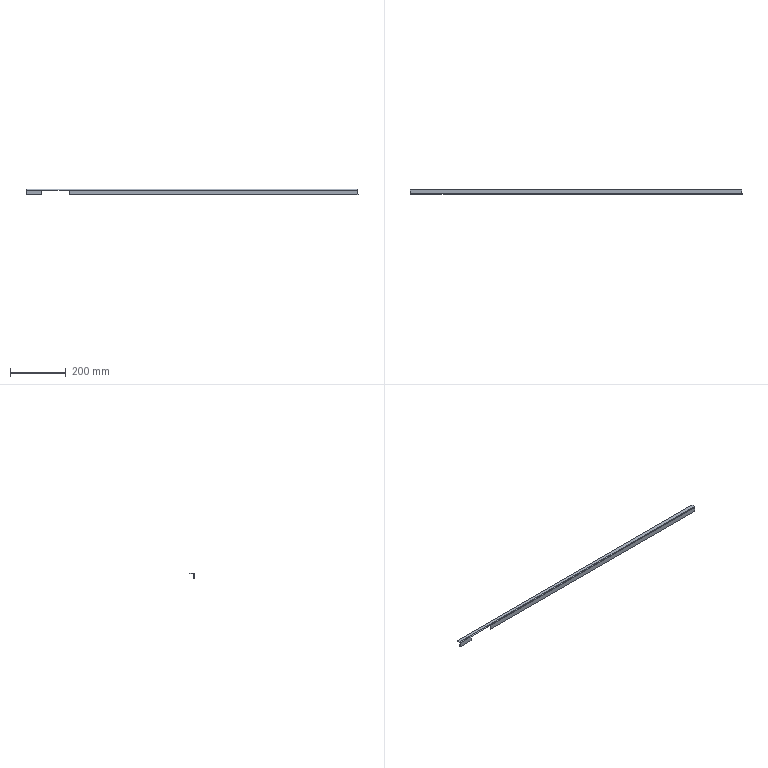Part | SolidWorks | features EdgeFlange 1, FlatPattern 1, ICE 1, SMBaseFlange 1, SheetMetal 1 | 1 solid | 20 faces | box 1191 x 15 x 20 mm | volume 90282 mm3 | plane 18 | cylinder 2 | commonest cylinder face diameters 1 x1 6 x1
STEP:
#1=CARTESIAN_POINT('',(595.5,-7.5,-3.));
#2=VERTEX_POINT('',#1);
#3=CARTESIAN_POINT('',(-440.,-7.5,-3.));
#4=VERTEX_POINT('',#3);
#5=CARTESIAN_POINT('',(-595.5,-7.5,-3.));
#6=DIRECTION('',(-1.,0.,0.));
#7=VECTOR('',#6,1000.);
#8=LINE('',#5,#7);
#9=EDGE_CURVE('',#2,#4,#8,.T.);
#10=ORIENTED_EDGE('',*,*,#9,.T.);
#11=CARTESIAN_POINT('',(-440.,-7.5,-20.));
#12=VERTEX_POINT('',#11);
#13=CARTESIAN_POINT('',(-440.,-7.5,-2.5));
#14=DIRECTION('',(0.,0.,-1.));
#15=VECTOR('',#14,1000.);
#16=LINE('',#13,#15);
#17=EDGE_CURVE('',#4,#12,#16,.T.);
#18=ORIENTED_EDGE('',*,*,#17,.T.);
#19=CARTESIAN_POINT('',(595.5,-7.5,-20.));
#20=VERTEX_POINT('',#19);
#21=CARTESIAN_POINT('',(-595.5,-7.5,-20.));
#22=DIRECTION('',(-1.,0.,0.));
#23=VECTOR('',#22,1000.);
#24=LINE('',#21,#23);
#25=EDGE_CURVE('',#20,#12,#24,.T.);
#26=ORIENTED_EDGE('',*,*,#25,.F.);
#27=CARTESIAN_POINT('',(595.5,-7.5,-20.));
#28=DIRECTION('',(0.,0.,-1.));
#29=VECTOR('',#28,1000.);
#30=LINE('',#27,#29);
#31=EDGE_CURVE('',#2,#20,#30,.T.);
#32=ORIENTED_EDGE('',*,*,#31,.F.);
#33=EDGE_LOOP('',(#10,#18,#26,#32));
#34=FACE_OUTER_BOUND('',#33,.T.);
#35=CARTESIAN_POINT('',(-595.5,-7.5,-2.5));
#36=DIRECTION('',(0.,-1.,0.));
#37=DIRECTION('',(0.,0.,-1.));
#38=AXIS2_PLACEMENT_3D('',#35,#36,#37);
#39=PLANE('',#38);
#40=ADVANCED_FACE('',(#34),#39,.T.);
#41=CARTESIAN_POINT('',(-540.,-7.5,-20.));
#42=VERTEX_POINT('',#41);
#43=CARTESIAN_POINT('',(-595.5,-7.5,-20.));
#44=VERTEX_POINT('',#43);
#45=CARTESIAN_POINT('',(-595.5,-7.5,-20.));
#46=DIRECTION('',(-1.,0.,0.));
#47=VECTOR('',#46,1000.);
#48=LINE('',#45,#47);
#49=EDGE_CURVE('',#42,#44,#48,.T.);
#50=ORIENTED_EDGE('',*,*,#49,.F.);
#51=CARTESIAN_POINT('',(-540.,-7.5,-3.));
#52=VERTEX_POINT('',#51);
#53=CARTESIAN_POINT('',(-540.,-7.5,-2.5));
#54=DIRECTION('',(0.,0.,1.));
#55=VECTOR('',#54,1000.);
#56=LINE('',#53,#55);
#57=EDGE_CURVE('',#42,#52,#56,.T.);
#58=ORIENTED_EDGE('',*,*,#57,.T.);
#59=CARTESIAN_POINT('',(-595.5,-7.5,-3.));
#60=VERTEX_POINT('',#59);
#61=CARTESIAN_POINT('',(-595.5,-7.5,-3.));
#62=DIRECTION('',(-1.,0.,0.));
#63=VECTOR('',#62,1000.);
#64=LINE('',#61,#63);
#65=EDGE_CURVE('',#52,#60,#64,.T.);
#66=ORIENTED_EDGE('',*,*,#65,.T.);
#67=CARTESIAN_POINT('',(-595.5,-7.5,-2.5));
#68=DIRECTION('',(0.,0.,1.));
#69=VECTOR('',#68,1000.);
#70=LINE('',#67,#69);
#71=EDGE_CURVE('',#44,#60,#70,.T.);
#72=ORIENTED_EDGE('',*,*,#71,.F.);
#73=EDGE_LOOP('',(#50,#58,#66,#72));
#74=FACE_OUTER_BOUND('',#73,.T.);
#75=CARTESIAN_POINT('',(-595.5,-7.5,-2.5));
#76=DIRECTION('',(0.,-1.,0.));
#77=DIRECTION('',(0.,0.,-1.));
#78=AXIS2_PLACEMENT_3D('',#75,#76,#77);
#79=PLANE('',#78);
#80=ADVANCED_FACE('',(#74),#79,.T.);
#81=CARTESIAN_POINT('',(-440.,-5.,-3.));
#82=VERTEX_POINT('',#81);
#83=CARTESIAN_POINT('',(-440.,-5.,-20.));
#84=VERTEX_POINT('',#83);
#85=CARTESIAN_POINT('',(-440.,-5.,-3.));
#86=DIRECTION('',(0.,0.,-1.));
#87=VECTOR('',#86,1000.);
#88=LINE('',#85,#87);
#89=EDGE_CURVE('',#82,#84,#88,.T.);
#90=ORIENTED_EDGE('',*,*,#89,.F.);
#91=CARTESIAN_POINT('',(595.5,-5.,-3.));
#92=VERTEX_POINT('',#91);
#93=CARTESIAN_POINT('',(595.5,-5.,-3.));
#94=DIRECTION('',(-1.,0.,0.));
#95=VECTOR('',#94,1000.);
#96=LINE('',#93,#95);
#97=EDGE_CURVE('',#92,#82,#96,.T.);
#98=ORIENTED_EDGE('',*,*,#97,.F.);
#99=CARTESIAN_POINT('',(595.5,-5.,-20.));
#100=VERTEX_POINT('',#99);
#101=CARTESIAN_POINT('',(595.5,-5.,-2.5));
#102=DIRECTION('',(0.,0.,-1.));
#103=VECTOR('',#102,1000.);
#104=LINE('',#101,#103);
#105=EDGE_CURVE('',#92,#100,#104,.T.);
#106=ORIENTED_EDGE('',*,*,#105,.T.);
#107=CARTESIAN_POINT('',(-595.5,-5.,-20.));
#108=DIRECTION('',(-1.,0.,0.));
#109=VECTOR('',#108,1000.);
#110=LINE('',#107,#109);
#111=EDGE_CURVE('',#100,#84,#110,.T.);
#112=ORIENTED_EDGE('',*,*,#111,.T.);
#113=EDGE_LOOP('',(#90,#98,#106,#112));
#114=FACE_OUTER_BOUND('',#113,.T.);
#115=CARTESIAN_POINT('',(-595.5,-5.,-2.5));
#116=DIRECTION('',(0.,-1.,0.));
#117=DIRECTION('',(0.,0.,-1.));
#118=AXIS2_PLACEMENT_3D('',#115,#116,#117);
#119=PLANE('',#118);
#120=ADVANCED_FACE('',(#114),#119,.F.);
#121=CARTESIAN_POINT('',(-540.,-5.,-20.));
#122=VERTEX_POINT('',#121);
#123=CARTESIAN_POINT('',(-540.,-5.,-3.));
#124=VERTEX_POINT('',#123);
#125=CARTESIAN_POINT('',(-540.,-5.,-3.));
#126=DIRECTION('',(0.,0.,1.));
#127=VECTOR('',#126,1000.);
#128=LINE('',#125,#127);
#129=EDGE_CURVE('',#122,#124,#128,.T.);
#130=ORIENTED_EDGE('',*,*,#129,.F.);
#131=CARTESIAN_POINT('',(-595.5,-5.,-20.));
#132=VERTEX_POINT('',#131);
#133=CARTESIAN_POINT('',(-595.5,-5.,-20.));
#134=DIRECTION('',(-1.,0.,0.));
#135=VECTOR('',#134,1000.);
#136=LINE('',#133,#135);
#137=EDGE_CURVE('',#122,#132,#136,.T.);
#138=ORIENTED_EDGE('',*,*,#137,.T.);
#139=CARTESIAN_POINT('',(-595.5,-5.,-3.));
#140=VERTEX_POINT('',#139);
#141=CARTESIAN_POINT('',(-595.5,-5.,-2.5));
#142=DIRECTION('',(0.,0.,1.));
#143=VECTOR('',#142,1000.);
#144=LINE('',#141,#143);
#145=EDGE_CURVE('',#132,#140,#144,.T.);
#146=ORIENTED_EDGE('',*,*,#145,.T.);
#147=CARTESIAN_POINT('',(595.5,-5.,-3.));
#148=DIRECTION('',(-1.,0.,0.));
#149=VECTOR('',#148,1000.);
#150=LINE('',#147,#149);
#151=EDGE_CURVE('',#124,#140,#150,.T.);
#152=ORIENTED_EDGE('',*,*,#151,.F.);
#153=EDGE_LOOP('',(#130,#138,#146,#152));
#154=FACE_OUTER_BOUND('',#153,.T.);
#155=CARTESIAN_POINT('',(-595.5,-5.,-2.5));
#156=DIRECTION('',(0.,-1.,0.));
#157=DIRECTION('',(0.,0.,-1.));
#158=AXIS2_PLACEMENT_3D('',#155,#156,#157);
#159=PLANE('',#158);
#160=ADVANCED_FACE('',(#154),#159,.F.);
#161=ORIENTED_EDGE('',*,*,#25,.T.);
#162=CARTESIAN_POINT('',(-440.,-5.,-20.));
#163=DIRECTION('',(0.,-1.,0.));
#164=VECTOR('',#163,1000.);
#165=LINE('',#162,#164);
#166=EDGE_CURVE('',#84,#12,#165,.T.);
#167=ORIENTED_EDGE('',*,*,#166,.F.);
#168=ORIENTED_EDGE('',*,*,#111,.F.);
#169=CARTESIAN_POINT('',(595.5,-7.5,-20.));
#170=DIRECTION('',(0.,1.,0.));
#171=VECTOR('',#170,1000.);
#172=LINE('',#169,#171);
#173=EDGE_CURVE('',#20,#100,#172,.T.);
#174=ORIENTED_EDGE('',*,*,#173,.F.);
#175=EDGE_LOOP('',(#161,#167,#168,#174));
#176=FACE_OUTER_BOUND('',#175,.T.);
#177=CARTESIAN_POINT('',(-595.5,-7.5,-20.));
#178=DIRECTION('',(0.,0.,-1.));
#179=DIRECTION('',(0.,1.,0.));
#180=AXIS2_PLACEMENT_3D('',#177,#178,#179);
#181=PLANE('',#180);
#182=ADVANCED_FACE('',(#176),#181,.T.);
#183=ORIENTED_EDGE('',*,*,#137,.F.);
#184=CARTESIAN_POINT('',(-540.,-5.,-20.));
#185=DIRECTION('',(0.,-1.,0.));
#186=VECTOR('',#185,1000.);
#187=LINE('',#184,#186);
#188=EDGE_CURVE('',#122,#42,#187,.T.);
#189=ORIENTED_EDGE('',*,*,#188,.T.);
#190=ORIENTED_EDGE('',*,*,#49,.T.);
#191=CARTESIAN_POINT('',(-595.5,-7.5,-20.));
#192=DIRECTION('',(0.,1.,0.));
#193=VECTOR('',#192,1000.);
#194=LINE('',#191,#193);
#195=EDGE_CURVE('',#44,#132,#194,.T.);
#196=ORIENTED_EDGE('',*,*,#195,.T.);
#197=EDGE_LOOP('',(#183,#189,#190,#196));
#198=FACE_OUTER_BOUND('',#197,.T.);
#199=CARTESIAN_POINT('',(-595.5,-7.5,-20.));
#200=DIRECTION('',(0.,0.,-1.));
#201=DIRECTION('',(0.,1.,0.));
#202=AXIS2_PLACEMENT_3D('',#199,#200,#201);
#203=PLANE('',#202);
#204=ADVANCED_FACE('',(#198),#203,.T.);
#205=CARTESIAN_POINT('',(-595.5,7.5,-2.5));
#206=VERTEX_POINT('',#205);
#207=CARTESIAN_POINT('',(-595.5,-4.5,-2.5));
#208=VERTEX_POINT('',#207);
#209=CARTESIAN_POINT('',(-595.5,-7.5,-2.5));
#210=DIRECTION('',(0.,-1.,0.));
#211=VECTOR('',#210,1000.);
#212=LINE('',#209,#211);
#213=EDGE_CURVE('',#206,#208,#212,.T.);
#214=ORIENTED_EDGE('',*,*,#213,.T.);
#215=CARTESIAN_POINT('',(-595.5,-4.5,0.));
#216=VERTEX_POINT('',#215);
#217=CARTESIAN_POINT('',(-595.5,-4.5,-2.5));
#218=DIRECTION('',(0.,0.,1.));
#219=VECTOR('',#218,1000.);
#220=LINE('',#217,#219);
#221=EDGE_CURVE('',#208,#216,#220,.T.);
#222=ORIENTED_EDGE('',*,*,#221,.T.);
#223=CARTESIAN_POINT('',(-595.5,7.5,0.));
#224=VERTEX_POINT('',#223);
#225=CARTESIAN_POINT('',(-595.5,-7.5,0.));
#226=DIRECTION('',(0.,-1.,0.));
#227=VECTOR('',#226,1000.);
#228=LINE('',#225,#227);
#229=EDGE_CURVE('',#224,#216,#228,.T.);
#230=ORIENTED_EDGE('',*,*,#229,.F.);
#231=CARTESIAN_POINT('',(-595.5,7.5,-2.5));
#232=DIRECTION('',(0.,0.,1.));
#233=VECTOR('',#232,1000.);
#234=LINE('',#231,#233);
#235=EDGE_CURVE('',#206,#224,#234,.T.);
#236=ORIENTED_EDGE('',*,*,#235,.F.);
#237=EDGE_LOOP('',(#214,#222,#230,#236));
#238=FACE_OUTER_BOUND('',#237,.T.);
#239=CARTESIAN_POINT('',(-595.5,-7.5,-2.5));
#240=DIRECTION('',(-1.,0.,0.));
#241=DIRECTION('',(0.,0.,1.));
#242=AXIS2_PLACEMENT_3D('',#239,#240,#241);
#243=PLANE('',#242);
#244=ADVANCED_FACE('',(#238),#243,.T.);
#245=CARTESIAN_POINT('',(595.5,-4.5,-2.5));
#246=VERTEX_POINT('',#245);
#247=CARTESIAN_POINT('',(595.5,7.5,-2.5));
#248=VERTEX_POINT('',#247);
#249=CARTESIAN_POINT('',(595.5,-7.5,-2.5));
#250=DIRECTION('',(0.,1.,0.));
#251=VECTOR('',#250,1000.);
#252=LINE('',#249,#251);
#253=EDGE_CURVE('',#246,#248,#252,.T.);
#254=ORIENTED_EDGE('',*,*,#253,.F.);
#255=CARTESIAN_POINT('',(-595.5,-4.5,-2.5));
#256=DIRECTION('',(1.,0.,0.));
#257=VECTOR('',#256,1000.);
#258=LINE('',#255,#257);
#259=EDGE_CURVE('',#208,#246,#258,.T.);
#260=ORIENTED_EDGE('',*,*,#259,.F.);
#261=ORIENTED_EDGE('',*,*,#213,.F.);
#262=CARTESIAN_POINT('',(-595.5,7.5,-2.5));
#263=DIRECTION('',(-1.,0.,0.));
#264=VECTOR('',#263,1000.);
#265=LINE('',#262,#264);
#266=EDGE_CURVE('',#248,#206,#265,.T.);
#267=ORIENTED_EDGE('',*,*,#266,.F.);
#268=EDGE_LOOP('',(#254,#260,#261,#267));
#269=FACE_OUTER_BOUND('',#268,.T.);
#270=CARTESIAN_POINT('',(595.5,7.5,-2.5));
#271=DIRECTION('',(0.,0.,-1.));
#272=DIRECTION('',(-1.,0.,0.));
#273=AXIS2_PLACEMENT_3D('',#270,#271,#272);
#274=PLANE('',#273);
#275=ADVANCED_FACE('',(#269),#274,.T.);
#276=CARTESIAN_POINT('',(595.5,-4.5,0.));
#277=VERTEX_POINT('',#276);
#278=CARTESIAN_POINT('',(-595.5,-4.5,0.));
#279=DIRECTION('',(1.,0.,0.));
#280=VECTOR('',#279,1000.);
#281=LINE('',#278,#280);
#282=EDGE_CURVE('',#216,#277,#281,.T.);
#283=ORIENTED_EDGE('',*,*,#282,.T.);
#284=CARTESIAN_POINT('',(595.5,7.5,0.));
#285=VERTEX_POINT('',#284);
#286=CARTESIAN_POINT('',(595.5,-7.5,0.));
#287=DIRECTION('',(0.,1.,0.));
#288=VECTOR('',#287,1000.);
#289=LINE('',#286,#288);
#290=EDGE_CURVE('',#277,#285,#289,.T.);
#291=ORIENTED_EDGE('',*,*,#290,.T.);
#292=CARTESIAN_POINT('',(-595.5,7.5,0.));
#293=DIRECTION('',(-1.,0.,0.));
#294=VECTOR('',#293,1000.);
#295=LINE('',#292,#294);
#296=EDGE_CURVE('',#285,#224,#295,.T.);
#297=ORIENTED_EDGE('',*,*,#296,.T.);
#298=ORIENTED_EDGE('',*,*,#229,.T.);
#299=EDGE_LOOP('',(#283,#291,#297,#298));
#300=FACE_OUTER_BOUND('',#299,.T.);
#301=CARTESIAN_POINT('',(595.5,7.5,0.));
#302=DIRECTION('',(0.,0.,-1.));
#303=DIRECTION('',(-1.,0.,0.));
#304=AXIS2_PLACEMENT_3D('',#301,#302,#303);
#305=PLANE('',#304);
#306=ADVANCED_FACE('',(#300),#305,.F.);
#307=CARTESIAN_POINT('',(595.5,-4.5,-2.5));
#308=DIRECTION('',(0.,0.,1.));
#309=VECTOR('',#308,1000.);
#310=LINE('',#307,#309);
#311=EDGE_CURVE('',#246,#277,#310,.T.);
#312=ORIENTED_EDGE('',*,*,#311,.F.);
#313=ORIENTED_EDGE('',*,*,#253,.T.);
#314=CARTESIAN_POINT('',(595.5,7.5,-2.5));
#315=DIRECTION('',(0.,0.,1.));
#316=VECTOR('',#315,1000.);
#317=LINE('',#314,#316);
#318=EDGE_CURVE('',#248,#285,#317,.T.);
#319=ORIENTED_EDGE('',*,*,#318,.T.);
#320=ORIENTED_EDGE('',*,*,#290,.F.);
#321=EDGE_LOOP('',(#312,#313,#319,#320));
#322=FACE_OUTER_BOUND('',#321,.T.);
#323=CARTESIAN_POINT('',(595.5,-7.5,-2.5));
#324=DIRECTION('',(1.,0.,0.));
#325=DIRECTION('',(0.,0.,-1.));
#326=AXIS2_PLACEMENT_3D('',#323,#324,#325);
#327=PLANE('',#326);
#328=ADVANCED_FACE('',(#322),#327,.T.);
#329=ORIENTED_EDGE('',*,*,#296,.F.);
#330=ORIENTED_EDGE('',*,*,#318,.F.);
#331=ORIENTED_EDGE('',*,*,#266,.T.);
#332=ORIENTED_EDGE('',*,*,#235,.T.);
#333=EDGE_LOOP('',(#329,#330,#331,#332));
#334=FACE_OUTER_BOUND('',#333,.T.);
#335=CARTESIAN_POINT('',(-595.5,7.5,-2.5));
#336=DIRECTION('',(0.,1.,0.));
#337=DIRECTION('',(0.,0.,1.));
#338=AXIS2_PLACEMENT_3D('',#335,#336,#337);
#339=PLANE('',#338);
#340=ADVANCED_FACE('',(#334),#339,.T.);
#341=CARTESIAN_POINT('',(595.5,-7.5,-3.));
#342=DIRECTION('',(0.,-1.,0.));
#343=VECTOR('',#342,1000.);
#344=LINE('',#341,#343);
#345=EDGE_CURVE('',#92,#2,#344,.T.);
#346=ORIENTED_EDGE('',*,*,#345,.F.);
#347=CARTESIAN_POINT('',(595.5,-4.5,-3.));
#348=DIRECTION('',(1.,0.,0.));
#349=DIRECTION('',(0.,0.,1.));
#350=AXIS2_PLACEMENT_3D('',#347,#348,#349);
#351=CIRCLE('',#350,0.5);
#352=EDGE_CURVE('',#246,#92,#351,.T.);
#353=ORIENTED_EDGE('',*,*,#352,.F.);
#354=ORIENTED_EDGE('',*,*,#311,.T.);
#355=CARTESIAN_POINT('',(595.5,-4.5,-3.));
#356=DIRECTION('',(1.,0.,0.));
#357=DIRECTION('',(0.,0.,1.));
#358=AXIS2_PLACEMENT_3D('',#355,#356,#357);
#359=CIRCLE('',#358,3.);
#360=EDGE_CURVE('',#277,#2,#359,.T.);
#361=ORIENTED_EDGE('',*,*,#360,.T.);
#362=EDGE_LOOP('',(#346,#353,#354,#361));
#363=FACE_OUTER_BOUND('',#362,.T.);
#364=CARTESIAN_POINT('',(595.5,-4.5,-3.));
#365=DIRECTION('',(1.,0.,0.));
#366=DIRECTION('',(0.,0.,-1.));
#367=AXIS2_PLACEMENT_3D('',#364,#365,#366);
#368=PLANE('',#367);
#369=ADVANCED_FACE('',(#363),#368,.T.);
#370=ORIENTED_EDGE('',*,*,#282,.F.);
#371=CARTESIAN_POINT('',(-595.5,-4.5,-3.));
#372=DIRECTION('',(-1.,0.,0.));
#373=DIRECTION('',(0.,0.,1.));
#374=AXIS2_PLACEMENT_3D('',#371,#372,#373);
#375=CIRCLE('',#374,3.);
#376=EDGE_CURVE('',#60,#216,#375,.T.);
#377=ORIENTED_EDGE('',*,*,#376,.F.);
#378=ORIENTED_EDGE('',*,*,#65,.F.);
#379=CARTESIAN_POINT('',(-595.5,-7.5,-3.));
#380=DIRECTION('',(1.,0.,0.));
#381=VECTOR('',#380,1000.);
#382=LINE('',#379,#381);
#383=EDGE_CURVE('',#52,#4,#382,.T.);
#384=ORIENTED_EDGE('',*,*,#383,.T.);
#385=ORIENTED_EDGE('',*,*,#9,.F.);
#386=ORIENTED_EDGE('',*,*,#360,.F.);
#387=EDGE_LOOP('',(#370,#377,#378,#384,#385,#386));
#388=FACE_OUTER_BOUND('',#387,.T.);
#389=CARTESIAN_POINT('',(-595.5,-4.5,-3.));
#390=DIRECTION('',(-1.,0.,0.));
#391=DIRECTION('',(0.,-1.,0.));
#392=AXIS2_PLACEMENT_3D('',#389,#390,#391);
#393=CYLINDRICAL_SURFACE('',#392,3.);
#394=ADVANCED_FACE('',(#388),#393,.T.);
#395=CARTESIAN_POINT('',(-595.5,-4.5,-3.));
#396=DIRECTION('',(-1.,0.,0.));
#397=DIRECTION('',(0.,0.,1.));
#398=AXIS2_PLACEMENT_3D('',#395,#396,#397);
#399=CIRCLE('',#398,0.5);
#400=EDGE_CURVE('',#140,#208,#399,.T.);
#401=ORIENTED_EDGE('',*,*,#400,.F.);
#402=CARTESIAN_POINT('',(-595.5,-5.,-3.));
#403=DIRECTION('',(0.,-1.,0.));
#404=VECTOR('',#403,1000.);
#405=LINE('',#402,#404);
#406=EDGE_CURVE('',#140,#60,#405,.T.);
#407=ORIENTED_EDGE('',*,*,#406,.T.);
#408=ORIENTED_EDGE('',*,*,#376,.T.);
#409=ORIENTED_EDGE('',*,*,#221,.F.);
#410=EDGE_LOOP('',(#401,#407,#408,#409));
#411=FACE_OUTER_BOUND('',#410,.T.);
#412=CARTESIAN_POINT('',(-595.5,-4.5,-3.));
#413=DIRECTION('',(1.,0.,0.));
#414=DIRECTION('',(0.,0.,-1.));
#415=AXIS2_PLACEMENT_3D('',#412,#413,#414);
#416=PLANE('',#415);
#417=ADVANCED_FACE('',(#411),#416,.F.);
#418=ORIENTED_EDGE('',*,*,#259,.T.);
#419=ORIENTED_EDGE('',*,*,#352,.T.);
#420=ORIENTED_EDGE('',*,*,#97,.T.);
#421=CARTESIAN_POINT('',(-540.,-5.,-3.));
#422=DIRECTION('',(1.,0.,0.));
#423=VECTOR('',#422,1000.);
#424=LINE('',#421,#423);
#425=EDGE_CURVE('',#124,#82,#424,.T.);
#426=ORIENTED_EDGE('',*,*,#425,.F.);
#427=ORIENTED_EDGE('',*,*,#151,.T.);
#428=ORIENTED_EDGE('',*,*,#400,.T.);
#429=EDGE_LOOP('',(#418,#419,#420,#426,#427,#428));
#430=FACE_OUTER_BOUND('',#429,.T.);
#431=CARTESIAN_POINT('',(-595.5,-4.5,-3.));
#432=DIRECTION('',(-1.,0.,0.));
#433=DIRECTION('',(0.,-1.,0.));
#434=AXIS2_PLACEMENT_3D('',#431,#432,#433);
#435=CYLINDRICAL_SURFACE('',#434,0.5);
#436=ADVANCED_FACE('',(#430),#435,.F.);
#437=ORIENTED_EDGE('',*,*,#71,.T.);
#438=ORIENTED_EDGE('',*,*,#406,.F.);
#439=ORIENTED_EDGE('',*,*,#145,.F.);
#440=ORIENTED_EDGE('',*,*,#195,.F.);
#441=EDGE_LOOP('',(#437,#438,#439,#440));
#442=FACE_OUTER_BOUND('',#441,.T.);
#443=CARTESIAN_POINT('',(-595.5,-7.5,-2.5));
#444=DIRECTION('',(-1.,0.,0.));
#445=DIRECTION('',(0.,0.,1.));
#446=AXIS2_PLACEMENT_3D('',#443,#444,#445);
#447=PLANE('',#446);
#448=ADVANCED_FACE('',(#442),#447,.T.);
#449=ORIENTED_EDGE('',*,*,#105,.F.);
#450=ORIENTED_EDGE('',*,*,#345,.T.);
#451=ORIENTED_EDGE('',*,*,#31,.T.);
#452=ORIENTED_EDGE('',*,*,#173,.T.);
#453=EDGE_LOOP('',(#449,#450,#451,#452));
#454=FACE_OUTER_BOUND('',#453,.T.);
#455=CARTESIAN_POINT('',(595.5,-7.5,-20.));
#456=DIRECTION('',(1.,0.,0.));
#457=DIRECTION('',(0.,0.,-1.));
#458=AXIS2_PLACEMENT_3D('',#455,#456,#457);
#459=PLANE('',#458);
#460=ADVANCED_FACE('',(#454),#459,.T.);
#461=CARTESIAN_POINT('',(-440.,-5.,-3.));
#462=DIRECTION('',(0.,-1.,0.));
#463=VECTOR('',#462,1000.);
#464=LINE('',#461,#463);
#465=EDGE_CURVE('',#82,#4,#464,.T.);
#466=ORIENTED_EDGE('',*,*,#465,.F.);
#467=ORIENTED_EDGE('',*,*,#89,.T.);
#468=ORIENTED_EDGE('',*,*,#166,.T.);
#469=ORIENTED_EDGE('',*,*,#17,.F.);
#470=EDGE_LOOP('',(#466,#467,#468,#469));
#471=FACE_OUTER_BOUND('',#470,.T.);
#472=CARTESIAN_POINT('',(-440.,-5.,-3.));
#473=DIRECTION('',(-1.,0.,0.));
#474=DIRECTION('',(0.,0.,-1.));
#475=AXIS2_PLACEMENT_3D('',#472,#473,#474);
#476=PLANE('',#475);
#477=ADVANCED_FACE('',(#471),#476,.T.);
#478=ORIENTED_EDGE('',*,*,#188,.F.);
#479=ORIENTED_EDGE('',*,*,#129,.T.);
#480=CARTESIAN_POINT('',(-540.,-5.,-3.));
#481=DIRECTION('',(0.,-1.,0.));
#482=VECTOR('',#481,1000.);
#483=LINE('',#480,#482);
#484=EDGE_CURVE('',#124,#52,#483,.T.);
#485=ORIENTED_EDGE('',*,*,#484,.T.);
#486=ORIENTED_EDGE('',*,*,#57,.F.);
#487=EDGE_LOOP('',(#478,#479,#485,#486));
#488=FACE_OUTER_BOUND('',#487,.T.);
#489=CARTESIAN_POINT('',(-540.,-5.,-3.));
#490=DIRECTION('',(1.,0.,0.));
#491=DIRECTION('',(0.,0.,1.));
#492=AXIS2_PLACEMENT_3D('',#489,#490,#491);
#493=PLANE('',#492);
#494=ADVANCED_FACE('',(#488),#493,.T.);
#495=ORIENTED_EDGE('',*,*,#425,.T.);
#496=ORIENTED_EDGE('',*,*,#465,.T.);
#497=ORIENTED_EDGE('',*,*,#383,.F.);
#498=ORIENTED_EDGE('',*,*,#484,.F.);
#499=EDGE_LOOP('',(#495,#496,#497,#498));
#500=FACE_OUTER_BOUND('',#499,.T.);
#501=CARTESIAN_POINT('',(-540.,-5.,-3.));
#502=DIRECTION('',(0.,0.,-1.));
#503=DIRECTION('',(1.,0.,0.));
#504=AXIS2_PLACEMENT_3D('',#501,#502,#503);
#505=PLANE('',#504);
#506=ADVANCED_FACE('',(#500),#505,.T.);
#507=CLOSED_SHELL('',(#40,#80,#120,#160,#182,#204,#244,#275,#306,#328,#340,#369,#394,#417,#436,#448,#460,#477,#494,#506));
#508=MANIFOLD_SOLID_BREP('',#507);
#509=CARTESIAN_POINT('',(0.,0.,0.));
#510=DIRECTION('',(0.,0.,1.));
#511=DIRECTION('',(1.,0.,0.));
#512=AXIS2_PLACEMENT_3D('',#509,#510,#511);
#513=(LENGTH_UNIT()NAMED_UNIT(*)SI_UNIT(.MILLI.,.METRE.));
#514=UNCERTAINTY_MEASURE_WITH_UNIT(LENGTH_MEASURE(0.00001),#513,'','');
#515=(NAMED_UNIT(*)PLANE_ANGLE_UNIT()SI_UNIT($,.RADIAN.));
#516=(NAMED_UNIT(*)SI_UNIT($,.STERADIAN.)SOLID_ANGLE_UNIT());
#517=(GEOMETRIC_REPRESENTATION_CONTEXT(3)GLOBAL_UNCERTAINTY_ASSIGNED_CONTEXT((#514))GLOBAL_UNIT_ASSIGNED_CONTEXT((#513,#515,#516))REPRESENTATION_CONTEXT('',''));
#518=ADVANCED_BREP_SHAPE_REPRESENTATION('',(#508,#512),#517);